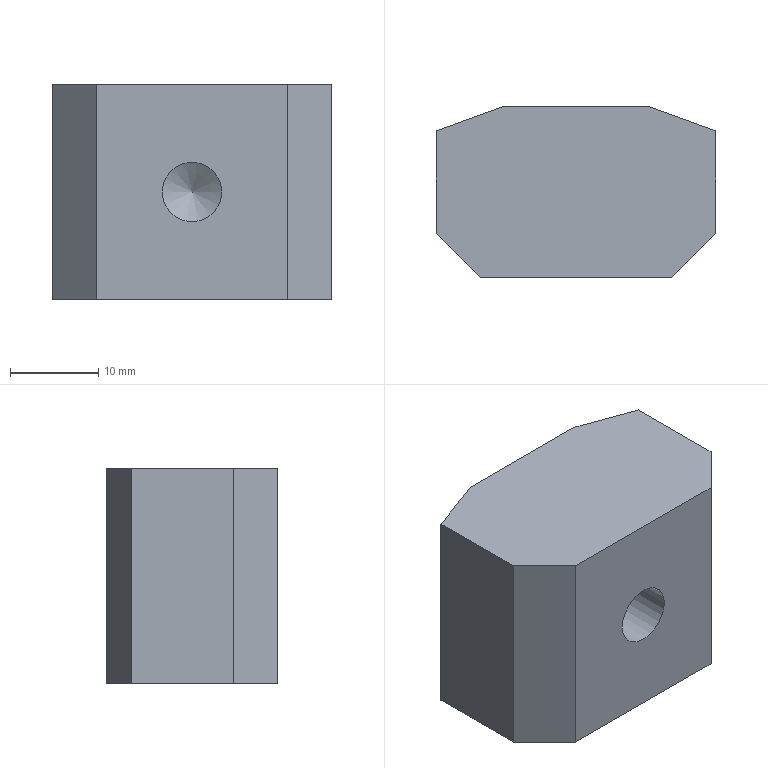Part | STEP file | 1_id1514_x_t | 1 solid | 12 faces | box 31.75 x 19.4 x 24.5 mm | volume 13370 mm3 | plane 10 | cone 1 | cylinder 1 | commonest cylinder face diameters 6.75 x1
STEP:
#1=CARTESIAN_POINT('',(0.,0.,0.));
#2=DIRECTION('',(0.,0.,1.));
#3=DIRECTION('',(1.,0.,0.));
#4=AXIS2_PLACEMENT_3D('',#1,#2,#3);
#5=CARTESIAN_POINT('',(42.476,77.647,12.25));
#6=VERTEX_POINT('',#5);
#7=CARTESIAN_POINT('',(49.226,77.647,12.25));
#8=VERTEX_POINT('',#7);
#9=CARTESIAN_POINT('',(45.851,77.647,12.25));
#10=DIRECTION('',(0.,-1.,0.));
#11=DIRECTION('',(1.,0.,0.));
#12=AXIS2_PLACEMENT_3D('',#9,#10,#11);
#13=CIRCLE('',#12,3.375);
#14=CARTESIAN_POINT('',(45.851,78.601,12.25));
#15=DIRECTION('',(0.,-1.,0.));
#16=DIRECTION('',(-1.,0.,0.));
#17=AXIS2_PLACEMENT_3D('',#14,#15,#16);
#18=CONICAL_SURFACE('',#17,1.721,1.047);
#19=CARTESIAN_POINT('',(-3.142,0.9548));
#20=DIRECTION('',(1.,0.));
#21=VECTOR('',#20,1.);
#22=LINE('',#19,#21);
#23=(GEOMETRIC_REPRESENTATION_CONTEXT(2)PARAMETRIC_REPRESENTATION_CONTEXT()REPRESENTATION_CONTEXT('',''));
#24=DEFINITIONAL_REPRESENTATION('',(#22),#23);
#25=PCURVE('',#18,#24);
#26=CARTESIAN_POINT('',(45.851,77.647,12.25));
#27=DIRECTION('',(0.,1.,0.));
#28=DIRECTION('',(-1.,0.,0.));
#29=AXIS2_PLACEMENT_3D('',#26,#27,#28);
#30=CYLINDRICAL_SURFACE('',#29,3.375);
#31=CARTESIAN_POINT('',(9.425,0.));
#32=DIRECTION('',(-1.,0.));
#33=VECTOR('',#32,1.);
#34=LINE('',#31,#33);
#35=(GEOMETRIC_REPRESENTATION_CONTEXT(2)PARAMETRIC_REPRESENTATION_CONTEXT()REPRESENTATION_CONTEXT('',''));
#36=DEFINITIONAL_REPRESENTATION('',(#34),#35);
#37=PCURVE('',#30,#36);
#38=SURFACE_CURVE('',#13,(#25,#37),.PCURVE_S1.);
#39=EDGE_CURVE('',#6,#8,#38,.T.);
#40=ORIENTED_EDGE('',*,*,#39,.F.);
#41=CARTESIAN_POINT('',(45.851,79.595,12.25));
#42=VERTEX_POINT('',#41);
#43=CARTESIAN_POINT('',(45.851,79.595,12.25));
#44=CARTESIAN_POINT('',(42.476,77.647,12.25));
#45=B_SPLINE_CURVE_WITH_KNOTS('',1,(#43,#44),.UNSPECIFIED.,.F.,.F.,(2,2),(-1.988,1.91),.PIECEWISE_BEZIER_KNOTS.);
#46=CARTESIAN_POINT('',(0.,0.));
#47=DIRECTION('',(0.,1.));
#48=VECTOR('',#47,1.);
#49=LINE('',#46,#48);
#50=(GEOMETRIC_REPRESENTATION_CONTEXT(2)PARAMETRIC_REPRESENTATION_CONTEXT()REPRESENTATION_CONTEXT('',''));
#51=DEFINITIONAL_REPRESENTATION('',(#49),#50);
#52=PCURVE('',#18,#51);
#53=CARTESIAN_POINT('',(6.283,0.));
#54=DIRECTION('',(0.,1.));
#55=VECTOR('',#54,1.);
#56=LINE('',#53,#55);
#57=(GEOMETRIC_REPRESENTATION_CONTEXT(2)PARAMETRIC_REPRESENTATION_CONTEXT()REPRESENTATION_CONTEXT('',''));
#58=DEFINITIONAL_REPRESENTATION('',(#56),#57);
#59=PCURVE('',#18,#58);
#60=SEAM_CURVE('',#45,(#52,#59),.PCURVE_S1.);
#61=EDGE_CURVE('',#42,#6,#60,.T.);
#62=ORIENTED_EDGE('',*,*,#61,.F.);
#63=ORIENTED_EDGE('',*,*,#61,.T.);
#64=CARTESIAN_POINT('',(45.851,77.647,12.25));
#65=DIRECTION('',(0.,-1.,0.));
#66=DIRECTION('',(1.,0.,0.));
#67=AXIS2_PLACEMENT_3D('',#64,#65,#66);
#68=CIRCLE('',#67,3.375);
#69=CARTESIAN_POINT('',(3.142,0.9548));
#70=DIRECTION('',(1.,0.));
#71=VECTOR('',#70,1.);
#72=LINE('',#69,#71);
#73=(GEOMETRIC_REPRESENTATION_CONTEXT(2)PARAMETRIC_REPRESENTATION_CONTEXT()REPRESENTATION_CONTEXT('',''));
#74=DEFINITIONAL_REPRESENTATION('',(#72),#73);
#75=PCURVE('',#18,#74);
#76=CARTESIAN_POINT('',(3.142,0.));
#77=DIRECTION('',(-1.,0.));
#78=VECTOR('',#77,1.);
#79=LINE('',#76,#78);
#80=(GEOMETRIC_REPRESENTATION_CONTEXT(2)PARAMETRIC_REPRESENTATION_CONTEXT()REPRESENTATION_CONTEXT('',''));
#81=DEFINITIONAL_REPRESENTATION('',(#79),#80);
#82=PCURVE('',#30,#81);
#83=SURFACE_CURVE('',#68,(#75,#82),.PCURVE_S1.);
#84=EDGE_CURVE('',#8,#6,#83,.T.);
#85=ORIENTED_EDGE('',*,*,#84,.F.);
#86=EDGE_LOOP('',(#40,#62,#63,#85));
#87=FACE_BOUND('',#86,.F.);
#88=ADVANCED_FACE('',(#87),#18,.F.);
#89=ORIENTED_EDGE('',*,*,#39,.T.);
#90=ORIENTED_EDGE('',*,*,#84,.T.);
#91=CARTESIAN_POINT('',(42.476,61.797,12.25));
#92=VERTEX_POINT('',#91);
#93=CARTESIAN_POINT('',(42.476,61.797,12.25));
#94=CARTESIAN_POINT('',(42.476,77.647,12.25));
#95=B_SPLINE_CURVE_WITH_KNOTS('',1,(#93,#94),.UNSPECIFIED.,.F.,.F.,(2,2),(-15.85,0.),.PIECEWISE_BEZIER_KNOTS.);
#96=CARTESIAN_POINT('',(0.,0.));
#97=DIRECTION('',(0.,1.));
#98=VECTOR('',#97,1.);
#99=LINE('',#96,#98);
#100=(GEOMETRIC_REPRESENTATION_CONTEXT(2)PARAMETRIC_REPRESENTATION_CONTEXT()REPRESENTATION_CONTEXT('',''));
#101=DEFINITIONAL_REPRESENTATION('',(#99),#100);
#102=PCURVE('',#30,#101);
#103=CARTESIAN_POINT('',(6.283,0.));
#104=DIRECTION('',(0.,1.));
#105=VECTOR('',#104,1.);
#106=LINE('',#103,#105);
#107=(GEOMETRIC_REPRESENTATION_CONTEXT(2)PARAMETRIC_REPRESENTATION_CONTEXT()REPRESENTATION_CONTEXT('',''));
#108=DEFINITIONAL_REPRESENTATION('',(#106),#107);
#109=PCURVE('',#30,#108);
#110=SEAM_CURVE('',#95,(#102,#109),.PCURVE_S1.);
#111=EDGE_CURVE('',#92,#6,#110,.T.);
#112=ORIENTED_EDGE('',*,*,#111,.F.);
#113=CARTESIAN_POINT('',(45.851,61.797,12.25));
#114=DIRECTION('',(0.,1.,0.));
#115=DIRECTION('',(-1.,0.,0.));
#116=AXIS2_PLACEMENT_3D('',#113,#114,#115);
#117=CIRCLE('',#116,3.375);
#118=CARTESIAN_POINT('',(0.,-15.85));
#119=DIRECTION('',(1.,0.));
#120=VECTOR('',#119,1.);
#121=LINE('',#118,#120);
#122=(GEOMETRIC_REPRESENTATION_CONTEXT(2)PARAMETRIC_REPRESENTATION_CONTEXT()REPRESENTATION_CONTEXT('',''));
#123=DEFINITIONAL_REPRESENTATION('',(#121),#122);
#124=PCURVE('',#30,#123);
#125=CARTESIAN_POINT('',(132.79,61.797,-25.177));
#126=DIRECTION('',(0.,-1.,0.));
#127=DIRECTION('',(-1.,0.,0.));
#128=AXIS2_PLACEMENT_3D('',#125,#126,#127);
#129=PLANE('',#128);
#130=CARTESIAN_POINT('',(90.314,-37.427));
#131=CARTESIAN_POINT('',(90.314,-43.273));
#132=CARTESIAN_POINT('',(85.252,-40.35));
#133=CARTESIAN_POINT('',(80.189,-37.427));
#134=CARTESIAN_POINT('',(85.252,-34.504));
#135=CARTESIAN_POINT('',(90.314,-31.581));
#136=CARTESIAN_POINT('',(90.314,-37.427));
#137=(BOUNDED_CURVE()B_SPLINE_CURVE(2,(#130,#131,#132,#133,#134,#135,#136),.UNSPECIFIED.,.T.,.F.)B_SPLINE_CURVE_WITH_KNOTS((1,2,2,2,2,1),(-2.094,0.,2.094,4.189,6.283,8.378),.UNSPECIFIED.)CURVE()GEOMETRIC_REPRESENTATION_ITEM()RATIONAL_B_SPLINE_CURVE((1.,0.5,1.,0.5,1.,0.5,1.))REPRESENTATION_ITEM(''));
#138=(GEOMETRIC_REPRESENTATION_CONTEXT(2)PARAMETRIC_REPRESENTATION_CONTEXT()REPRESENTATION_CONTEXT('',''));
#139=DEFINITIONAL_REPRESENTATION('',(#137),#138);
#140=PCURVE('',#129,#139);
#141=SURFACE_CURVE('',#117,(#124,#140),.PCURVE_S1.);
#142=EDGE_CURVE('',#92,#92,#141,.T.);
#143=ORIENTED_EDGE('',*,*,#142,.T.);
#144=ORIENTED_EDGE('',*,*,#111,.T.);
#145=EDGE_LOOP('',(#89,#90,#112,#143,#144));
#146=FACE_BOUND('',#145,.F.);
#147=ADVANCED_FACE('',(#146),#30,.F.);
#148=CARTESIAN_POINT('',(34.976,61.797,24.5));
#149=VERTEX_POINT('',#148);
#150=CARTESIAN_POINT('',(34.976,61.797,0.));
#151=VERTEX_POINT('',#150);
#152=CARTESIAN_POINT('',(34.976,61.797,24.5));
#153=DIRECTION('',(0.,0.,-1.));
#154=VECTOR('',#153,1.);
#155=LINE('',#152,#154);
#156=CARTESIAN_POINT('',(97.814,-49.677));
#157=DIRECTION('',(0.,1.));
#158=VECTOR('',#157,1.);
#159=LINE('',#156,#158);
#160=(GEOMETRIC_REPRESENTATION_CONTEXT(2)PARAMETRIC_REPRESENTATION_CONTEXT()REPRESENTATION_CONTEXT('',''));
#161=DEFINITIONAL_REPRESENTATION('',(#159),#160);
#162=PCURVE('',#129,#161);
#163=CARTESIAN_POINT('',(29.976,66.797,0.1));
#164=DIRECTION('',(0.7071,0.7071,0.));
#165=DIRECTION('',(0.,0.,1.));
#166=AXIS2_PLACEMENT_3D('',#163,#164,#165);
#167=PLANE('',#166);
#168=CARTESIAN_POINT('',(24.4,7.071));
#169=DIRECTION('',(-1.,0.));
#170=VECTOR('',#169,1.);
#171=LINE('',#168,#170);
#172=(GEOMETRIC_REPRESENTATION_CONTEXT(2)PARAMETRIC_REPRESENTATION_CONTEXT()REPRESENTATION_CONTEXT('',''));
#173=DEFINITIONAL_REPRESENTATION('',(#171),#172);
#174=PCURVE('',#167,#173);
#175=SURFACE_CURVE('',#155,(#162,#174),.PCURVE_S1.);
#176=EDGE_CURVE('',#149,#151,#175,.T.);
#177=ORIENTED_EDGE('',*,*,#176,.T.);
#178=CARTESIAN_POINT('',(56.726,61.797,0.));
#179=VERTEX_POINT('',#178);
#180=CARTESIAN_POINT('',(34.976,61.797,0.));
#181=DIRECTION('',(1.,0.,0.));
#182=VECTOR('',#181,1.);
#183=LINE('',#180,#182);
#184=CARTESIAN_POINT('',(97.814,-25.177));
#185=DIRECTION('',(-1.,0.));
#186=VECTOR('',#185,1.);
#187=LINE('',#184,#186);
#188=(GEOMETRIC_REPRESENTATION_CONTEXT(2)PARAMETRIC_REPRESENTATION_CONTEXT()REPRESENTATION_CONTEXT('',''));
#189=DEFINITIONAL_REPRESENTATION('',(#187),#188);
#190=PCURVE('',#129,#189);
#191=CARTESIAN_POINT('',(275.801,29.473,0.));
#192=DIRECTION('',(0.,0.,-1.));
#193=DIRECTION('',(0.,-1.,0.));
#194=AXIS2_PLACEMENT_3D('',#191,#192,#193);
#195=PLANE('',#194);
#196=CARTESIAN_POINT('',(-32.324,240.825));
#197=DIRECTION('',(0.,-1.));
#198=VECTOR('',#197,1.);
#199=LINE('',#196,#198);
#200=(GEOMETRIC_REPRESENTATION_CONTEXT(2)PARAMETRIC_REPRESENTATION_CONTEXT()REPRESENTATION_CONTEXT('',''));
#201=DEFINITIONAL_REPRESENTATION('',(#199),#200);
#202=PCURVE('',#195,#201);
#203=SURFACE_CURVE('',#183,(#190,#202),.PCURVE_S1.);
#204=EDGE_CURVE('',#151,#179,#203,.T.);
#205=ORIENTED_EDGE('',*,*,#204,.T.);
#206=CARTESIAN_POINT('',(56.726,61.797,24.5));
#207=VERTEX_POINT('',#206);
#208=CARTESIAN_POINT('',(56.726,61.797,0.));
#209=DIRECTION('',(0.,0.,1.));
#210=VECTOR('',#209,1.);
#211=LINE('',#208,#210);
#212=CARTESIAN_POINT('',(76.064,-25.177));
#213=DIRECTION('',(0.,-1.));
#214=VECTOR('',#213,1.);
#215=LINE('',#212,#214);
#216=(GEOMETRIC_REPRESENTATION_CONTEXT(2)PARAMETRIC_REPRESENTATION_CONTEXT()REPRESENTATION_CONTEXT('',''));
#217=DEFINITIONAL_REPRESENTATION('',(#215),#216);
#218=PCURVE('',#129,#217);
#219=CARTESIAN_POINT('',(61.726,66.797,0.1));
#220=DIRECTION('',(-0.7071,0.7071,0.));
#221=DIRECTION('',(0.7071,0.7071,0.));
#222=AXIS2_PLACEMENT_3D('',#219,#220,#221);
#223=PLANE('',#222);
#224=CARTESIAN_POINT('',(-7.071,0.1));
#225=DIRECTION('',(0.,-1.));
#226=VECTOR('',#225,1.);
#227=LINE('',#224,#226);
#228=(GEOMETRIC_REPRESENTATION_CONTEXT(2)PARAMETRIC_REPRESENTATION_CONTEXT()REPRESENTATION_CONTEXT('',''));
#229=DEFINITIONAL_REPRESENTATION('',(#227),#228);
#230=PCURVE('',#223,#229);
#231=SURFACE_CURVE('',#211,(#218,#230),.PCURVE_S1.);
#232=EDGE_CURVE('',#179,#207,#231,.T.);
#233=ORIENTED_EDGE('',*,*,#232,.T.);
#234=CARTESIAN_POINT('',(34.976,61.797,24.5));
#235=DIRECTION('',(1.,0.,0.));
#236=VECTOR('',#235,1.);
#237=LINE('',#234,#236);
#238=CARTESIAN_POINT('',(97.814,-49.677));
#239=DIRECTION('',(-1.,0.));
#240=VECTOR('',#239,1.);
#241=LINE('',#238,#240);
#242=(GEOMETRIC_REPRESENTATION_CONTEXT(2)PARAMETRIC_REPRESENTATION_CONTEXT()REPRESENTATION_CONTEXT('',''));
#243=DEFINITIONAL_REPRESENTATION('',(#241),#242);
#244=PCURVE('',#129,#243);
#245=CARTESIAN_POINT('',(280.801,31.977,24.5));
#246=DIRECTION('',(0.,0.,1.));
#247=DIRECTION('',(-1.,0.,0.));
#248=AXIS2_PLACEMENT_3D('',#245,#246,#247);
#249=PLANE('',#248);
#250=CARTESIAN_POINT('',(245.825,-29.82));
#251=DIRECTION('',(-1.,0.));
#252=VECTOR('',#251,1.);
#253=LINE('',#250,#252);
#254=(GEOMETRIC_REPRESENTATION_CONTEXT(2)PARAMETRIC_REPRESENTATION_CONTEXT()REPRESENTATION_CONTEXT('',''));
#255=DEFINITIONAL_REPRESENTATION('',(#253),#254);
#256=PCURVE('',#249,#255);
#257=SURFACE_CURVE('',#237,(#244,#256),.PCURVE_S1.);
#258=EDGE_CURVE('',#149,#207,#257,.T.);
#259=ORIENTED_EDGE('',*,*,#258,.F.);
#260=EDGE_LOOP('',(#177,#205,#233,#259));
#261=FACE_BOUND('',#260,.T.);
#262=ORIENTED_EDGE('',*,*,#142,.T.);
#263=EDGE_LOOP('',(#262));
#264=FACE_BOUND('',#263,.T.);
#265=ADVANCED_FACE('',(#261,#264),#129,.T.);
#266=CARTESIAN_POINT('',(61.726,78.423,24.5));
#267=VERTEX_POINT('',#266);
#268=CARTESIAN_POINT('',(54.106,81.197,24.5));
#269=VERTEX_POINT('',#268);
#270=CARTESIAN_POINT('',(61.726,78.423,24.5));
#271=DIRECTION('',(-0.9397,0.342,0.));
#272=VECTOR('',#271,1.);
#273=LINE('',#270,#272);
#274=CARTESIAN_POINT('',(219.075,-46.447));
#275=DIRECTION('',(0.9397,-0.342));
#276=VECTOR('',#275,1.);
#277=LINE('',#274,#276);
#278=(GEOMETRIC_REPRESENTATION_CONTEXT(2)PARAMETRIC_REPRESENTATION_CONTEXT()REPRESENTATION_CONTEXT('',''));
#279=DEFINITIONAL_REPRESENTATION('',(#277),#278);
#280=PCURVE('',#249,#279);
#281=CARTESIAN_POINT('',(61.726,78.423,0.1));
#282=DIRECTION('',(0.342,0.9397,0.));
#283=DIRECTION('',(0.,0.,1.));
#284=AXIS2_PLACEMENT_3D('',#281,#282,#283);
#285=PLANE('',#284);
#286=CARTESIAN_POINT('',(24.4,0.));
#287=DIRECTION('',(0.,-1.));
#288=VECTOR('',#287,1.);
#289=LINE('',#286,#288);
#290=(GEOMETRIC_REPRESENTATION_CONTEXT(2)PARAMETRIC_REPRESENTATION_CONTEXT()REPRESENTATION_CONTEXT('',''));
#291=DEFINITIONAL_REPRESENTATION('',(#289),#290);
#292=PCURVE('',#285,#291);
#293=SURFACE_CURVE('',#273,(#280,#292),.PCURVE_S1.);
#294=EDGE_CURVE('',#267,#269,#293,.T.);
#295=ORIENTED_EDGE('',*,*,#294,.T.);
#296=CARTESIAN_POINT('',(37.596,81.197,24.5));
#297=VERTEX_POINT('',#296);
#298=CARTESIAN_POINT('',(37.596,81.197,24.5));
#299=DIRECTION('',(1.,0.,0.));
#300=VECTOR('',#299,1.);
#301=LINE('',#298,#300);
#302=CARTESIAN_POINT('',(243.205,-49.22));
#303=DIRECTION('',(-1.,0.));
#304=VECTOR('',#303,1.);
#305=LINE('',#302,#304);
#306=(GEOMETRIC_REPRESENTATION_CONTEXT(2)PARAMETRIC_REPRESENTATION_CONTEXT()REPRESENTATION_CONTEXT('',''));
#307=DEFINITIONAL_REPRESENTATION('',(#305),#306);
#308=PCURVE('',#249,#307);
#309=CARTESIAN_POINT('',(54.106,81.197,0.1));
#310=DIRECTION('',(0.,1.,0.));
#311=DIRECTION('',(0.,0.,1.));
#312=AXIS2_PLACEMENT_3D('',#309,#310,#311);
#313=PLANE('',#312);
#314=CARTESIAN_POINT('',(24.4,-16.51));
#315=DIRECTION('',(0.,1.));
#316=VECTOR('',#315,1.);
#317=LINE('',#314,#316);
#318=(GEOMETRIC_REPRESENTATION_CONTEXT(2)PARAMETRIC_REPRESENTATION_CONTEXT()REPRESENTATION_CONTEXT('',''));
#319=DEFINITIONAL_REPRESENTATION('',(#317),#318);
#320=PCURVE('',#313,#319);
#321=SURFACE_CURVE('',#301,(#308,#320),.PCURVE_S1.);
#322=EDGE_CURVE('',#297,#269,#321,.T.);
#323=ORIENTED_EDGE('',*,*,#322,.F.);
#324=CARTESIAN_POINT('',(29.976,78.423,24.5));
#325=VERTEX_POINT('',#324);
#326=CARTESIAN_POINT('',(37.596,81.197,24.5));
#327=DIRECTION('',(-0.9397,-0.342,0.));
#328=VECTOR('',#327,1.);
#329=LINE('',#326,#328);
#330=CARTESIAN_POINT('',(243.205,-49.22));
#331=DIRECTION('',(0.9397,0.342));
#332=VECTOR('',#331,1.);
#333=LINE('',#330,#332);
#334=(GEOMETRIC_REPRESENTATION_CONTEXT(2)PARAMETRIC_REPRESENTATION_CONTEXT()REPRESENTATION_CONTEXT('',''));
#335=DEFINITIONAL_REPRESENTATION('',(#333),#334);
#336=PCURVE('',#249,#335);
#337=CARTESIAN_POINT('',(37.596,81.197,0.1));
#338=DIRECTION('',(-0.342,0.9397,0.));
#339=DIRECTION('',(0.9397,0.342,0.));
#340=AXIS2_PLACEMENT_3D('',#337,#338,#339);
#341=PLANE('',#340);
#342=CARTESIAN_POINT('',(0.,-24.4));
#343=DIRECTION('',(-1.,0.));
#344=VECTOR('',#343,1.);
#345=LINE('',#342,#344);
#346=(GEOMETRIC_REPRESENTATION_CONTEXT(2)PARAMETRIC_REPRESENTATION_CONTEXT()REPRESENTATION_CONTEXT('',''));
#347=DEFINITIONAL_REPRESENTATION('',(#345),#346);
#348=PCURVE('',#341,#347);
#349=SURFACE_CURVE('',#329,(#336,#348),.PCURVE_S1.);
#350=EDGE_CURVE('',#297,#325,#349,.T.);
#351=ORIENTED_EDGE('',*,*,#350,.T.);
#352=CARTESIAN_POINT('',(29.976,66.797,24.5));
#353=VERTEX_POINT('',#352);
#354=CARTESIAN_POINT('',(29.976,66.797,24.5));
#355=DIRECTION('',(0.,1.,0.));
#356=VECTOR('',#355,1.);
#357=LINE('',#354,#356);
#358=CARTESIAN_POINT('',(250.825,-34.82));
#359=DIRECTION('',(0.,-1.));
#360=VECTOR('',#359,1.);
#361=LINE('',#358,#360);
#362=(GEOMETRIC_REPRESENTATION_CONTEXT(2)PARAMETRIC_REPRESENTATION_CONTEXT()REPRESENTATION_CONTEXT('',''));
#363=DEFINITIONAL_REPRESENTATION('',(#361),#362);
#364=PCURVE('',#249,#363);
#365=CARTESIAN_POINT('',(29.976,79.023,0.1));
#366=DIRECTION('',(-1.,0.,0.));
#367=DIRECTION('',(0.,1.,0.));
#368=AXIS2_PLACEMENT_3D('',#365,#366,#367);
#369=PLANE('',#368);
#370=CARTESIAN_POINT('',(-12.227,-24.4));
#371=DIRECTION('',(1.,0.));
#372=VECTOR('',#371,1.);
#373=LINE('',#370,#372);
#374=(GEOMETRIC_REPRESENTATION_CONTEXT(2)PARAMETRIC_REPRESENTATION_CONTEXT()REPRESENTATION_CONTEXT('',''));
#375=DEFINITIONAL_REPRESENTATION('',(#373),#374);
#376=PCURVE('',#369,#375);
#377=SURFACE_CURVE('',#357,(#364,#376),.PCURVE_S1.);
#378=EDGE_CURVE('',#353,#325,#377,.T.);
#379=ORIENTED_EDGE('',*,*,#378,.F.);
#380=CARTESIAN_POINT('',(29.976,66.797,24.5));
#381=DIRECTION('',(0.7071,-0.7071,0.));
#382=VECTOR('',#381,1.);
#383=LINE('',#380,#382);
#384=CARTESIAN_POINT('',(250.825,-34.82));
#385=DIRECTION('',(-0.7071,0.7071));
#386=VECTOR('',#385,1.);
#387=LINE('',#384,#386);
#388=(GEOMETRIC_REPRESENTATION_CONTEXT(2)PARAMETRIC_REPRESENTATION_CONTEXT()REPRESENTATION_CONTEXT('',''));
#389=DEFINITIONAL_REPRESENTATION('',(#387),#388);
#390=PCURVE('',#249,#389);
#391=CARTESIAN_POINT('',(24.4,0.));
#392=DIRECTION('',(0.,1.));
#393=VECTOR('',#392,1.);
#394=LINE('',#391,#393);
#395=(GEOMETRIC_REPRESENTATION_CONTEXT(2)PARAMETRIC_REPRESENTATION_CONTEXT()REPRESENTATION_CONTEXT('',''));
#396=DEFINITIONAL_REPRESENTATION('',(#394),#395);
#397=PCURVE('',#167,#396);
#398=SURFACE_CURVE('',#383,(#390,#397),.PCURVE_S1.);
#399=EDGE_CURVE('',#353,#149,#398,.T.);
#400=ORIENTED_EDGE('',*,*,#399,.T.);
#401=ORIENTED_EDGE('',*,*,#258,.T.);
#402=CARTESIAN_POINT('',(61.726,66.797,24.5));
#403=VERTEX_POINT('',#402);
#404=CARTESIAN_POINT('',(56.726,61.797,24.5));
#405=DIRECTION('',(0.7071,0.7071,0.));
#406=VECTOR('',#405,1.);
#407=LINE('',#404,#406);
#408=CARTESIAN_POINT('',(224.075,-29.82));
#409=DIRECTION('',(-0.7071,-0.7071));
#410=VECTOR('',#409,1.);
#411=LINE('',#408,#410);
#412=(GEOMETRIC_REPRESENTATION_CONTEXT(2)PARAMETRIC_REPRESENTATION_CONTEXT()REPRESENTATION_CONTEXT('',''));
#413=DEFINITIONAL_REPRESENTATION('',(#411),#412);
#414=PCURVE('',#249,#413);
#415=CARTESIAN_POINT('',(-7.071,-24.4));
#416=DIRECTION('',(1.,0.));
#417=VECTOR('',#416,1.);
#418=LINE('',#415,#417);
#419=(GEOMETRIC_REPRESENTATION_CONTEXT(2)PARAMETRIC_REPRESENTATION_CONTEXT()REPRESENTATION_CONTEXT('',''));
#420=DEFINITIONAL_REPRESENTATION('',(#418),#419);
#421=PCURVE('',#223,#420);
#422=SURFACE_CURVE('',#407,(#414,#421),.PCURVE_S1.);
#423=EDGE_CURVE('',#207,#403,#422,.T.);
#424=ORIENTED_EDGE('',*,*,#423,.T.);
#425=CARTESIAN_POINT('',(61.726,78.423,24.5));
#426=DIRECTION('',(0.,-1.,0.));
#427=VECTOR('',#426,1.);
#428=LINE('',#425,#427);
#429=CARTESIAN_POINT('',(219.075,-46.447));
#430=DIRECTION('',(0.,1.));
#431=VECTOR('',#430,1.);
#432=LINE('',#429,#431);
#433=(GEOMETRIC_REPRESENTATION_CONTEXT(2)PARAMETRIC_REPRESENTATION_CONTEXT()REPRESENTATION_CONTEXT('',''));
#434=DEFINITIONAL_REPRESENTATION('',(#432),#433);
#435=PCURVE('',#249,#434);
#436=CARTESIAN_POINT('',(61.726,54.873,0.1));
#437=DIRECTION('',(1.,0.,0.));
#438=DIRECTION('',(0.,1.,0.));
#439=AXIS2_PLACEMENT_3D('',#436,#437,#438);
#440=PLANE('',#439);
#441=CARTESIAN_POINT('',(23.551,24.4));
#442=DIRECTION('',(-1.,0.));
#443=VECTOR('',#442,1.);
#444=LINE('',#441,#443);
#445=(GEOMETRIC_REPRESENTATION_CONTEXT(2)PARAMETRIC_REPRESENTATION_CONTEXT()REPRESENTATION_CONTEXT('',''));
#446=DEFINITIONAL_REPRESENTATION('',(#444),#445);
#447=PCURVE('',#440,#446);
#448=SURFACE_CURVE('',#428,(#435,#447),.PCURVE_S1.);
#449=EDGE_CURVE('',#267,#403,#448,.T.);
#450=ORIENTED_EDGE('',*,*,#449,.F.);
#451=EDGE_LOOP('',(#295,#323,#351,#379,#400,#401,#424,#450));
#452=FACE_BOUND('',#451,.T.);
#453=ADVANCED_FACE('',(#452),#249,.T.);
#454=CARTESIAN_POINT('',(61.726,78.423,0.));
#455=VERTEX_POINT('',#454);
#456=CARTESIAN_POINT('',(61.726,78.423,24.5));
#457=DIRECTION('',(0.,0.,-1.));
#458=VECTOR('',#457,1.);
#459=LINE('',#456,#458);
#460=CARTESIAN_POINT('',(23.551,24.4));
#461=DIRECTION('',(0.,-1.));
#462=VECTOR('',#461,1.);
#463=LINE('',#460,#462);
#464=(GEOMETRIC_REPRESENTATION_CONTEXT(2)PARAMETRIC_REPRESENTATION_CONTEXT()REPRESENTATION_CONTEXT('',''));
#465=DEFINITIONAL_REPRESENTATION('',(#463),#464);
#466=PCURVE('',#440,#465);
#467=CARTESIAN_POINT('',(24.4,0.));
#468=DIRECTION('',(-1.,0.));
#469=VECTOR('',#468,1.);
#470=LINE('',#467,#469);
#471=(GEOMETRIC_REPRESENTATION_CONTEXT(2)PARAMETRIC_REPRESENTATION_CONTEXT()REPRESENTATION_CONTEXT('',''));
#472=DEFINITIONAL_REPRESENTATION('',(#470),#471);
#473=PCURVE('',#285,#472);
#474=SURFACE_CURVE('',#459,(#466,#473),.PCURVE_S1.);
#475=EDGE_CURVE('',#267,#455,#474,.T.);
#476=ORIENTED_EDGE('',*,*,#475,.F.);
#477=ORIENTED_EDGE('',*,*,#449,.T.);
#478=CARTESIAN_POINT('',(61.726,66.797,0.));
#479=VERTEX_POINT('',#478);
#480=CARTESIAN_POINT('',(61.726,66.797,24.5));
#481=DIRECTION('',(0.,0.,-1.));
#482=VECTOR('',#481,1.);
#483=LINE('',#480,#482);
#484=CARTESIAN_POINT('',(11.924,24.4));
#485=DIRECTION('',(0.,-1.));
#486=VECTOR('',#485,1.);
#487=LINE('',#484,#486);
#488=(GEOMETRIC_REPRESENTATION_CONTEXT(2)PARAMETRIC_REPRESENTATION_CONTEXT()REPRESENTATION_CONTEXT('',''));
#489=DEFINITIONAL_REPRESENTATION('',(#487),#488);
#490=PCURVE('',#440,#489);
#491=CARTESIAN_POINT('',(0.,-24.4));
#492=DIRECTION('',(0.,1.));
#493=VECTOR('',#492,1.);
#494=LINE('',#491,#493);
#495=(GEOMETRIC_REPRESENTATION_CONTEXT(2)PARAMETRIC_REPRESENTATION_CONTEXT()REPRESENTATION_CONTEXT('',''));
#496=DEFINITIONAL_REPRESENTATION('',(#494),#495);
#497=PCURVE('',#223,#496);
#498=SURFACE_CURVE('',#483,(#490,#497),.PCURVE_S1.);
#499=EDGE_CURVE('',#403,#479,#498,.T.);
#500=ORIENTED_EDGE('',*,*,#499,.T.);
#501=CARTESIAN_POINT('',(61.726,78.423,0.));
#502=DIRECTION('',(0.,-1.,0.));
#503=VECTOR('',#502,1.);
#504=LINE('',#501,#503);
#505=CARTESIAN_POINT('',(23.551,-0.1));
#506=DIRECTION('',(-1.,0.));
#507=VECTOR('',#506,1.);
#508=LINE('',#505,#507);
#509=(GEOMETRIC_REPRESENTATION_CONTEXT(2)PARAMETRIC_REPRESENTATION_CONTEXT()REPRESENTATION_CONTEXT('',''));
#510=DEFINITIONAL_REPRESENTATION('',(#508),#509);
#511=PCURVE('',#440,#510);
#512=CARTESIAN_POINT('',(-48.951,214.075));
#513=DIRECTION('',(1.,0.));
#514=VECTOR('',#513,1.);
#515=LINE('',#512,#514);
#516=(GEOMETRIC_REPRESENTATION_CONTEXT(2)PARAMETRIC_REPRESENTATION_CONTEXT()REPRESENTATION_CONTEXT('',''));
#517=DEFINITIONAL_REPRESENTATION('',(#515),#516);
#518=PCURVE('',#195,#517);
#519=SURFACE_CURVE('',#504,(#511,#518),.PCURVE_S1.);
#520=EDGE_CURVE('',#455,#479,#519,.T.);
#521=ORIENTED_EDGE('',*,*,#520,.F.);
#522=EDGE_LOOP('',(#476,#477,#500,#521));
#523=FACE_BOUND('',#522,.T.);
#524=ADVANCED_FACE('',(#523),#440,.T.);
#525=CARTESIAN_POINT('',(29.976,66.797,0.));
#526=VERTEX_POINT('',#525);
#527=CARTESIAN_POINT('',(34.976,61.797,0.));
#528=DIRECTION('',(-0.7071,0.7071,0.));
#529=VECTOR('',#528,1.);
#530=LINE('',#527,#529);
#531=CARTESIAN_POINT('',(-32.324,240.825));
#532=DIRECTION('',(-0.7071,0.7071));
#533=VECTOR('',#532,1.);
#534=LINE('',#531,#533);
#535=(GEOMETRIC_REPRESENTATION_CONTEXT(2)PARAMETRIC_REPRESENTATION_CONTEXT()REPRESENTATION_CONTEXT('',''));
#536=DEFINITIONAL_REPRESENTATION('',(#534),#535);
#537=PCURVE('',#195,#536);
#538=CARTESIAN_POINT('',(-0.1,7.071));
#539=DIRECTION('',(0.,-1.));
#540=VECTOR('',#539,1.);
#541=LINE('',#538,#540);
#542=(GEOMETRIC_REPRESENTATION_CONTEXT(2)PARAMETRIC_REPRESENTATION_CONTEXT()REPRESENTATION_CONTEXT('',''));
#543=DEFINITIONAL_REPRESENTATION('',(#541),#542);
#544=PCURVE('',#167,#543);
#545=SURFACE_CURVE('',#530,(#537,#544),.PCURVE_S1.);
#546=EDGE_CURVE('',#151,#526,#545,.T.);
#547=ORIENTED_EDGE('',*,*,#546,.T.);
#548=CARTESIAN_POINT('',(29.976,78.423,0.));
#549=VERTEX_POINT('',#548);
#550=CARTESIAN_POINT('',(29.976,66.797,0.));
#551=DIRECTION('',(0.,1.,0.));
#552=VECTOR('',#551,1.);
#553=LINE('',#550,#552);
#554=CARTESIAN_POINT('',(-37.324,245.825));
#555=DIRECTION('',(-1.,0.));
#556=VECTOR('',#555,1.);
#557=LINE('',#554,#556);
#558=(GEOMETRIC_REPRESENTATION_CONTEXT(2)PARAMETRIC_REPRESENTATION_CONTEXT()REPRESENTATION_CONTEXT('',''));
#559=DEFINITIONAL_REPRESENTATION('',(#557),#558);
#560=PCURVE('',#195,#559);
#561=CARTESIAN_POINT('',(-12.227,0.1));
#562=DIRECTION('',(1.,0.));
#563=VECTOR('',#562,1.);
#564=LINE('',#561,#563);
#565=(GEOMETRIC_REPRESENTATION_CONTEXT(2)PARAMETRIC_REPRESENTATION_CONTEXT()REPRESENTATION_CONTEXT('',''));
#566=DEFINITIONAL_REPRESENTATION('',(#564),#565);
#567=PCURVE('',#369,#566);
#568=SURFACE_CURVE('',#553,(#560,#567),.PCURVE_S1.);
#569=EDGE_CURVE('',#526,#549,#568,.T.);
#570=ORIENTED_EDGE('',*,*,#569,.T.);
#571=CARTESIAN_POINT('',(37.596,81.197,0.));
#572=VERTEX_POINT('',#571);
#573=CARTESIAN_POINT('',(29.976,78.423,0.));
#574=DIRECTION('',(0.9397,0.342,0.));
#575=VECTOR('',#574,1.);
#576=LINE('',#573,#575);
#577=CARTESIAN_POINT('',(-48.951,245.825));
#578=DIRECTION('',(-0.342,-0.9397));
#579=VECTOR('',#578,1.);
#580=LINE('',#577,#579);
#581=(GEOMETRIC_REPRESENTATION_CONTEXT(2)PARAMETRIC_REPRESENTATION_CONTEXT()REPRESENTATION_CONTEXT('',''));
#582=DEFINITIONAL_REPRESENTATION('',(#580),#581);
#583=PCURVE('',#195,#582);
#584=CARTESIAN_POINT('',(-8.109,0.1));
#585=DIRECTION('',(1.,0.));
#586=VECTOR('',#585,1.);
#587=LINE('',#584,#586);
#588=(GEOMETRIC_REPRESENTATION_CONTEXT(2)PARAMETRIC_REPRESENTATION_CONTEXT()REPRESENTATION_CONTEXT('',''));
#589=DEFINITIONAL_REPRESENTATION('',(#587),#588);
#590=PCURVE('',#341,#589);
#591=SURFACE_CURVE('',#576,(#583,#590),.PCURVE_S1.);
#592=EDGE_CURVE('',#549,#572,#591,.T.);
#593=ORIENTED_EDGE('',*,*,#592,.T.);
#594=CARTESIAN_POINT('',(54.106,81.197,0.));
#595=VERTEX_POINT('',#594);
#596=CARTESIAN_POINT('',(37.596,81.197,0.));
#597=DIRECTION('',(1.,0.,0.));
#598=VECTOR('',#597,1.);
#599=LINE('',#596,#598);
#600=CARTESIAN_POINT('',(-51.724,238.205));
#601=DIRECTION('',(0.,-1.));
#602=VECTOR('',#601,1.);
#603=LINE('',#600,#602);
#604=(GEOMETRIC_REPRESENTATION_CONTEXT(2)PARAMETRIC_REPRESENTATION_CONTEXT()REPRESENTATION_CONTEXT('',''));
#605=DEFINITIONAL_REPRESENTATION('',(#603),#604);
#606=PCURVE('',#195,#605);
#607=CARTESIAN_POINT('',(-0.1,-16.51));
#608=DIRECTION('',(0.,1.));
#609=VECTOR('',#608,1.);
#610=LINE('',#607,#609);
#611=(GEOMETRIC_REPRESENTATION_CONTEXT(2)PARAMETRIC_REPRESENTATION_CONTEXT()REPRESENTATION_CONTEXT('',''));
#612=DEFINITIONAL_REPRESENTATION('',(#610),#611);
#613=PCURVE('',#313,#612);
#614=SURFACE_CURVE('',#599,(#606,#613),.PCURVE_S1.);
#615=EDGE_CURVE('',#572,#595,#614,.T.);
#616=ORIENTED_EDGE('',*,*,#615,.T.);
#617=CARTESIAN_POINT('',(54.106,81.197,0.));
#618=DIRECTION('',(0.9397,-0.342,0.));
#619=VECTOR('',#618,1.);
#620=LINE('',#617,#619);
#621=CARTESIAN_POINT('',(-51.724,221.695));
#622=DIRECTION('',(0.342,-0.9397));
#623=VECTOR('',#622,1.);
#624=LINE('',#621,#623);
#625=(GEOMETRIC_REPRESENTATION_CONTEXT(2)PARAMETRIC_REPRESENTATION_CONTEXT()REPRESENTATION_CONTEXT('',''));
#626=DEFINITIONAL_REPRESENTATION('',(#624),#625);
#627=PCURVE('',#195,#626);
#628=CARTESIAN_POINT('',(-0.1,-8.109));
#629=DIRECTION('',(0.,1.));
#630=VECTOR('',#629,1.);
#631=LINE('',#628,#630);
#632=(GEOMETRIC_REPRESENTATION_CONTEXT(2)PARAMETRIC_REPRESENTATION_CONTEXT()REPRESENTATION_CONTEXT('',''));
#633=DEFINITIONAL_REPRESENTATION('',(#631),#632);
#634=PCURVE('',#285,#633);
#635=SURFACE_CURVE('',#620,(#627,#634),.PCURVE_S1.);
#636=EDGE_CURVE('',#595,#455,#635,.T.);
#637=ORIENTED_EDGE('',*,*,#636,.T.);
#638=ORIENTED_EDGE('',*,*,#520,.T.);
#639=CARTESIAN_POINT('',(61.726,66.797,0.));
#640=DIRECTION('',(-0.7071,-0.7071,0.));
#641=VECTOR('',#640,1.);
#642=LINE('',#639,#641);
#643=CARTESIAN_POINT('',(-37.324,214.075));
#644=DIRECTION('',(0.7071,0.7071));
#645=VECTOR('',#644,1.);
#646=LINE('',#643,#645);
#647=(GEOMETRIC_REPRESENTATION_CONTEXT(2)PARAMETRIC_REPRESENTATION_CONTEXT()REPRESENTATION_CONTEXT('',''));
#648=DEFINITIONAL_REPRESENTATION('',(#646),#647);
#649=PCURVE('',#195,#648);
#650=CARTESIAN_POINT('',(0.,0.1));
#651=DIRECTION('',(-1.,0.));
#652=VECTOR('',#651,1.);
#653=LINE('',#650,#652);
#654=(GEOMETRIC_REPRESENTATION_CONTEXT(2)PARAMETRIC_REPRESENTATION_CONTEXT()REPRESENTATION_CONTEXT('',''));
#655=DEFINITIONAL_REPRESENTATION('',(#653),#654);
#656=PCURVE('',#223,#655);
#657=SURFACE_CURVE('',#642,(#649,#656),.PCURVE_S1.);
#658=EDGE_CURVE('',#479,#179,#657,.T.);
#659=ORIENTED_EDGE('',*,*,#658,.T.);
#660=ORIENTED_EDGE('',*,*,#204,.F.);
#661=EDGE_LOOP('',(#547,#570,#593,#616,#637,#638,#659,#660));
#662=FACE_BOUND('',#661,.T.);
#663=ADVANCED_FACE('',(#662),#195,.T.);
#664=ORIENTED_EDGE('',*,*,#499,.F.);
#665=ORIENTED_EDGE('',*,*,#423,.F.);
#666=ORIENTED_EDGE('',*,*,#232,.F.);
#667=ORIENTED_EDGE('',*,*,#658,.F.);
#668=EDGE_LOOP('',(#664,#665,#666,#667));
#669=FACE_BOUND('',#668,.T.);
#670=ADVANCED_FACE('',(#669),#223,.F.);
#671=ORIENTED_EDGE('',*,*,#475,.T.);
#672=ORIENTED_EDGE('',*,*,#636,.F.);
#673=CARTESIAN_POINT('',(54.106,81.197,24.5));
#674=DIRECTION('',(0.,0.,-1.));
#675=VECTOR('',#674,1.);
#676=LINE('',#673,#675);
#677=CARTESIAN_POINT('',(24.4,-8.109));
#678=DIRECTION('',(-1.,0.));
#679=VECTOR('',#678,1.);
#680=LINE('',#677,#679);
#681=(GEOMETRIC_REPRESENTATION_CONTEXT(2)PARAMETRIC_REPRESENTATION_CONTEXT()REPRESENTATION_CONTEXT('',''));
#682=DEFINITIONAL_REPRESENTATION('',(#680),#681);
#683=PCURVE('',#285,#682);
#684=CARTESIAN_POINT('',(24.4,0.));
#685=DIRECTION('',(-1.,0.));
#686=VECTOR('',#685,1.);
#687=LINE('',#684,#686);
#688=(GEOMETRIC_REPRESENTATION_CONTEXT(2)PARAMETRIC_REPRESENTATION_CONTEXT()REPRESENTATION_CONTEXT('',''));
#689=DEFINITIONAL_REPRESENTATION('',(#687),#688);
#690=PCURVE('',#313,#689);
#691=SURFACE_CURVE('',#676,(#683,#690),.PCURVE_S1.);
#692=EDGE_CURVE('',#269,#595,#691,.T.);
#693=ORIENTED_EDGE('',*,*,#692,.F.);
#694=ORIENTED_EDGE('',*,*,#294,.F.);
#695=EDGE_LOOP('',(#671,#672,#693,#694));
#696=FACE_BOUND('',#695,.T.);
#697=ADVANCED_FACE('',(#696),#285,.T.);
#698=ORIENTED_EDGE('',*,*,#692,.T.);
#699=ORIENTED_EDGE('',*,*,#615,.F.);
#700=CARTESIAN_POINT('',(37.596,81.197,24.5));
#701=DIRECTION('',(0.,0.,-1.));
#702=VECTOR('',#701,1.);
#703=LINE('',#700,#702);
#704=CARTESIAN_POINT('',(24.4,-16.51));
#705=DIRECTION('',(-1.,0.));
#706=VECTOR('',#705,1.);
#707=LINE('',#704,#706);
#708=(GEOMETRIC_REPRESENTATION_CONTEXT(2)PARAMETRIC_REPRESENTATION_CONTEXT()REPRESENTATION_CONTEXT('',''));
#709=DEFINITIONAL_REPRESENTATION('',(#707),#708);
#710=PCURVE('',#313,#709);
#711=CARTESIAN_POINT('',(0.,-24.4));
#712=DIRECTION('',(0.,1.));
#713=VECTOR('',#712,1.);
#714=LINE('',#711,#713);
#715=(GEOMETRIC_REPRESENTATION_CONTEXT(2)PARAMETRIC_REPRESENTATION_CONTEXT()REPRESENTATION_CONTEXT('',''));
#716=DEFINITIONAL_REPRESENTATION('',(#714),#715);
#717=PCURVE('',#341,#716);
#718=SURFACE_CURVE('',#703,(#710,#717),.PCURVE_S1.);
#719=EDGE_CURVE('',#297,#572,#718,.T.);
#720=ORIENTED_EDGE('',*,*,#719,.F.);
#721=ORIENTED_EDGE('',*,*,#322,.T.);
#722=EDGE_LOOP('',(#698,#699,#720,#721));
#723=FACE_BOUND('',#722,.T.);
#724=ADVANCED_FACE('',(#723),#313,.T.);
#725=ORIENTED_EDGE('',*,*,#719,.T.);
#726=ORIENTED_EDGE('',*,*,#592,.F.);
#727=CARTESIAN_POINT('',(29.976,78.423,24.5));
#728=DIRECTION('',(0.,0.,-1.));
#729=VECTOR('',#728,1.);
#730=LINE('',#727,#729);
#731=CARTESIAN_POINT('',(-8.109,-24.4));
#732=DIRECTION('',(0.,1.));
#733=VECTOR('',#732,1.);
#734=LINE('',#731,#733);
#735=(GEOMETRIC_REPRESENTATION_CONTEXT(2)PARAMETRIC_REPRESENTATION_CONTEXT()REPRESENTATION_CONTEXT('',''));
#736=DEFINITIONAL_REPRESENTATION('',(#734),#735);
#737=PCURVE('',#341,#736);
#738=CARTESIAN_POINT('',(-0.6,-24.4));
#739=DIRECTION('',(0.,1.));
#740=VECTOR('',#739,1.);
#741=LINE('',#738,#740);
#742=(GEOMETRIC_REPRESENTATION_CONTEXT(2)PARAMETRIC_REPRESENTATION_CONTEXT()REPRESENTATION_CONTEXT('',''));
#743=DEFINITIONAL_REPRESENTATION('',(#741),#742);
#744=PCURVE('',#369,#743);
#745=SURFACE_CURVE('',#730,(#737,#744),.PCURVE_S1.);
#746=EDGE_CURVE('',#325,#549,#745,.T.);
#747=ORIENTED_EDGE('',*,*,#746,.F.);
#748=ORIENTED_EDGE('',*,*,#350,.F.);
#749=EDGE_LOOP('',(#725,#726,#747,#748));
#750=FACE_BOUND('',#749,.T.);
#751=ADVANCED_FACE('',(#750),#341,.T.);
#752=ORIENTED_EDGE('',*,*,#746,.T.);
#753=ORIENTED_EDGE('',*,*,#569,.F.);
#754=CARTESIAN_POINT('',(29.976,66.797,0.));
#755=DIRECTION('',(0.,0.,1.));
#756=VECTOR('',#755,1.);
#757=LINE('',#754,#756);
#758=CARTESIAN_POINT('',(-12.227,0.1));
#759=DIRECTION('',(0.,-1.));
#760=VECTOR('',#759,1.);
#761=LINE('',#758,#760);
#762=(GEOMETRIC_REPRESENTATION_CONTEXT(2)PARAMETRIC_REPRESENTATION_CONTEXT()REPRESENTATION_CONTEXT('',''));
#763=DEFINITIONAL_REPRESENTATION('',(#761),#762);
#764=PCURVE('',#369,#763);
#765=CARTESIAN_POINT('',(-0.1,0.));
#766=DIRECTION('',(1.,0.));
#767=VECTOR('',#766,1.);
#768=LINE('',#765,#767);
#769=(GEOMETRIC_REPRESENTATION_CONTEXT(2)PARAMETRIC_REPRESENTATION_CONTEXT()REPRESENTATION_CONTEXT('',''));
#770=DEFINITIONAL_REPRESENTATION('',(#768),#769);
#771=PCURVE('',#167,#770);
#772=SURFACE_CURVE('',#757,(#764,#771),.PCURVE_S1.);
#773=EDGE_CURVE('',#526,#353,#772,.T.);
#774=ORIENTED_EDGE('',*,*,#773,.T.);
#775=ORIENTED_EDGE('',*,*,#378,.T.);
#776=EDGE_LOOP('',(#752,#753,#774,#775));
#777=FACE_BOUND('',#776,.T.);
#778=ADVANCED_FACE('',(#777),#369,.T.);
#779=ORIENTED_EDGE('',*,*,#773,.F.);
#780=ORIENTED_EDGE('',*,*,#546,.F.);
#781=ORIENTED_EDGE('',*,*,#176,.F.);
#782=ORIENTED_EDGE('',*,*,#399,.F.);
#783=EDGE_LOOP('',(#779,#780,#781,#782));
#784=FACE_BOUND('',#783,.T.);
#785=ADVANCED_FACE('',(#784),#167,.F.);
#786=CLOSED_SHELL('',(#88,#147,#265,#453,#524,#663,#670,#697,#724,#751,#778,#785));
#787=MANIFOLD_SOLID_BREP('',#786);
#788=(LENGTH_UNIT()NAMED_UNIT(*)SI_UNIT(.MILLI.,.METRE.));
#789=UNCERTAINTY_MEASURE_WITH_UNIT(LENGTH_MEASURE(0.000001),#788,'','');
#790=(NAMED_UNIT(*)PLANE_ANGLE_UNIT()SI_UNIT($,.RADIAN.));
#791=(NAMED_UNIT(*)SI_UNIT($,.STERADIAN.)SOLID_ANGLE_UNIT());
#792=(GEOMETRIC_REPRESENTATION_CONTEXT(3)GLOBAL_UNCERTAINTY_ASSIGNED_CONTEXT((#789))GLOBAL_UNIT_ASSIGNED_CONTEXT((#788,#790,#791))REPRESENTATION_CONTEXT('',''));
#793=ADVANCED_BREP_SHAPE_REPRESENTATION('',(#4,#787),#792);